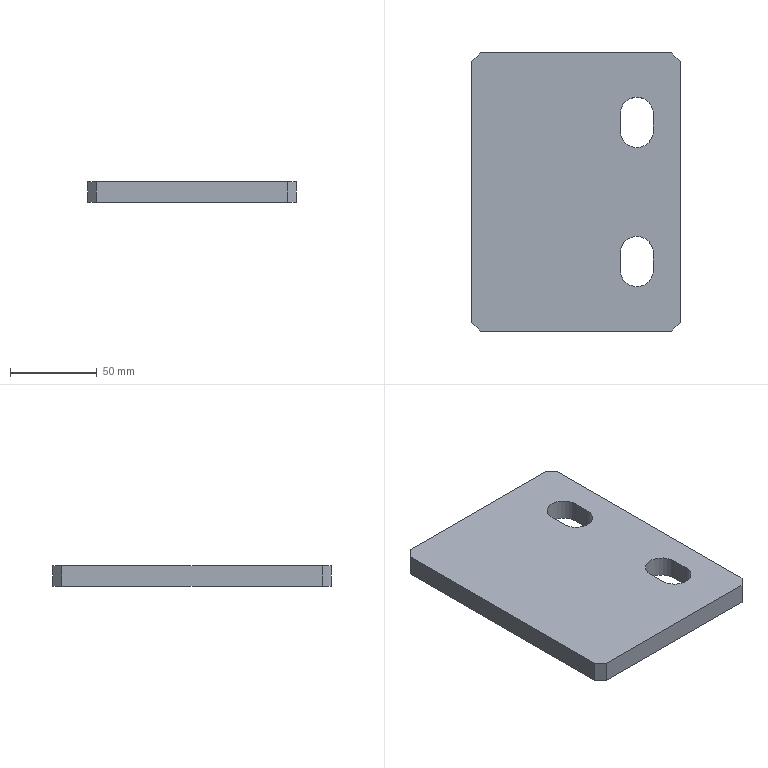Part | STEP file | Mirror_楼梯连接Plate 11 | 1 solid | 18 faces | box 120 x 160 x 12 mm | volume 218435 mm3 | plane 14 | cylinder 4 | commonest cylinder face diameters 19 x4
STEP:
#1=CARTESIAN_POINT('',(0.,0.,0.));
#2=DIRECTION('',(0.,0.,1.));
#3=DIRECTION('',(1.,0.,0.));
#4=AXIS2_PLACEMENT_3D('',#1,#2,#3);
#5=CARTESIAN_POINT('',(-60.,155.,0.));
#6=VERTEX_POINT('',#5);
#7=CARTESIAN_POINT('',(-60.,5.,0.));
#8=VERTEX_POINT('',#7);
#9=CARTESIAN_POINT('',(-60.,160.,0.));
#10=DIRECTION('',(0.,-1.,0.));
#11=VECTOR('',#10,1.);
#12=LINE('',#9,#11);
#13=CARTESIAN_POINT('',(-60.,160.,-12.));
#14=DIRECTION('',(1.,0.,0.));
#15=DIRECTION('',(0.,1.,0.));
#16=AXIS2_PLACEMENT_3D('',#13,#14,#15);
#17=PLANE('',#16);
#18=CARTESIAN_POINT('',(0.,12.));
#19=DIRECTION('',(-1.,0.));
#20=VECTOR('',#19,1.);
#21=LINE('',#18,#20);
#22=(GEOMETRIC_REPRESENTATION_CONTEXT(2)PARAMETRIC_REPRESENTATION_CONTEXT()REPRESENTATION_CONTEXT('',''));
#23=DEFINITIONAL_REPRESENTATION('',(#21),#22);
#24=PCURVE('',#17,#23);
#25=CARTESIAN_POINT('',(0.,0.,0.));
#26=DIRECTION('',(0.,0.,-1.));
#27=DIRECTION('',(1.,0.,0.));
#28=AXIS2_PLACEMENT_3D('',#25,#26,#27);
#29=PLANE('',#28);
#30=CARTESIAN_POINT('',(-60.,-160.));
#31=DIRECTION('',(0.,1.));
#32=VECTOR('',#31,1.);
#33=LINE('',#30,#32);
#34=(GEOMETRIC_REPRESENTATION_CONTEXT(2)PARAMETRIC_REPRESENTATION_CONTEXT()REPRESENTATION_CONTEXT('',''));
#35=DEFINITIONAL_REPRESENTATION('',(#33),#34);
#36=PCURVE('',#29,#35);
#37=SURFACE_CURVE('',#12,(#24,#36),.PCURVE_S1.);
#38=EDGE_CURVE('',#6,#8,#37,.T.);
#39=ORIENTED_EDGE('',*,*,#38,.F.);
#40=CARTESIAN_POINT('',(-60.,155.,-12.));
#41=VERTEX_POINT('',#40);
#42=CARTESIAN_POINT('',(-60.,155.,-12.));
#43=DIRECTION('',(0.,0.,1.));
#44=VECTOR('',#43,1.);
#45=LINE('',#42,#44);
#46=CARTESIAN_POINT('',(-5.,0.));
#47=DIRECTION('',(0.,1.));
#48=VECTOR('',#47,1.);
#49=LINE('',#46,#48);
#50=(GEOMETRIC_REPRESENTATION_CONTEXT(2)PARAMETRIC_REPRESENTATION_CONTEXT()REPRESENTATION_CONTEXT('',''));
#51=DEFINITIONAL_REPRESENTATION('',(#49),#50);
#52=PCURVE('',#17,#51);
#53=CARTESIAN_POINT('',(-60.,155.,-12.));
#54=DIRECTION('',(0.7071,-0.7071,0.));
#55=DIRECTION('',(0.,0.,1.));
#56=AXIS2_PLACEMENT_3D('',#53,#54,#55);
#57=PLANE('',#56);
#58=CARTESIAN_POINT('',(0.,0.));
#59=DIRECTION('',(1.,0.));
#60=VECTOR('',#59,1.);
#61=LINE('',#58,#60);
#62=(GEOMETRIC_REPRESENTATION_CONTEXT(2)PARAMETRIC_REPRESENTATION_CONTEXT()REPRESENTATION_CONTEXT('',''));
#63=DEFINITIONAL_REPRESENTATION('',(#61),#62);
#64=PCURVE('',#57,#63);
#65=SURFACE_CURVE('',#45,(#52,#64),.PCURVE_S1.);
#66=EDGE_CURVE('',#41,#6,#65,.T.);
#67=ORIENTED_EDGE('',*,*,#66,.F.);
#68=CARTESIAN_POINT('',(-60.,5.,-12.));
#69=VERTEX_POINT('',#68);
#70=CARTESIAN_POINT('',(-60.,160.,-12.));
#71=DIRECTION('',(0.,-1.,0.));
#72=VECTOR('',#71,1.);
#73=LINE('',#70,#72);
#74=CARTESIAN_POINT('',(0.,0.));
#75=DIRECTION('',(-1.,0.));
#76=VECTOR('',#75,1.);
#77=LINE('',#74,#76);
#78=(GEOMETRIC_REPRESENTATION_CONTEXT(2)PARAMETRIC_REPRESENTATION_CONTEXT()REPRESENTATION_CONTEXT('',''));
#79=DEFINITIONAL_REPRESENTATION('',(#77),#78);
#80=PCURVE('',#17,#79);
#81=CARTESIAN_POINT('',(0.,0.,-12.));
#82=DIRECTION('',(0.,0.,-1.));
#83=DIRECTION('',(1.,0.,0.));
#84=AXIS2_PLACEMENT_3D('',#81,#82,#83);
#85=PLANE('',#84);
#86=CARTESIAN_POINT('',(-60.,-160.));
#87=DIRECTION('',(0.,1.));
#88=VECTOR('',#87,1.);
#89=LINE('',#86,#88);
#90=(GEOMETRIC_REPRESENTATION_CONTEXT(2)PARAMETRIC_REPRESENTATION_CONTEXT()REPRESENTATION_CONTEXT('',''));
#91=DEFINITIONAL_REPRESENTATION('',(#89),#90);
#92=PCURVE('',#85,#91);
#93=SURFACE_CURVE('',#73,(#80,#92),.PCURVE_S1.);
#94=EDGE_CURVE('',#41,#69,#93,.T.);
#95=ORIENTED_EDGE('',*,*,#94,.T.);
#96=CARTESIAN_POINT('',(-60.,5.,-12.));
#97=DIRECTION('',(0.,0.,-1.));
#98=VECTOR('',#97,1.);
#99=LINE('',#96,#98);
#100=CARTESIAN_POINT('',(-155.,0.));
#101=DIRECTION('',(0.,-1.));
#102=VECTOR('',#101,1.);
#103=LINE('',#100,#102);
#104=(GEOMETRIC_REPRESENTATION_CONTEXT(2)PARAMETRIC_REPRESENTATION_CONTEXT()REPRESENTATION_CONTEXT('',''));
#105=DEFINITIONAL_REPRESENTATION('',(#103),#104);
#106=PCURVE('',#17,#105);
#107=CARTESIAN_POINT('',(-55.,0.,-12.));
#108=DIRECTION('',(0.7071,0.7071,0.));
#109=DIRECTION('',(0.,0.,1.));
#110=AXIS2_PLACEMENT_3D('',#107,#108,#109);
#111=PLANE('',#110);
#112=CARTESIAN_POINT('',(0.,-7.071));
#113=DIRECTION('',(-1.,0.));
#114=VECTOR('',#113,1.);
#115=LINE('',#112,#114);
#116=(GEOMETRIC_REPRESENTATION_CONTEXT(2)PARAMETRIC_REPRESENTATION_CONTEXT()REPRESENTATION_CONTEXT('',''));
#117=DEFINITIONAL_REPRESENTATION('',(#115),#116);
#118=PCURVE('',#111,#117);
#119=SURFACE_CURVE('',#99,(#106,#118),.PCURVE_S1.);
#120=EDGE_CURVE('',#8,#69,#119,.T.);
#121=ORIENTED_EDGE('',*,*,#120,.F.);
#122=EDGE_LOOP('',(#39,#67,#95,#121));
#123=FACE_BOUND('',#122,.T.);
#124=ADVANCED_FACE('',(#123),#17,.F.);
#125=CARTESIAN_POINT('',(-55.,0.,-12.));
#126=VERTEX_POINT('',#125);
#127=CARTESIAN_POINT('',(55.,0.,-12.));
#128=VERTEX_POINT('',#127);
#129=CARTESIAN_POINT('',(-60.,0.,-12.));
#130=DIRECTION('',(1.,0.,0.));
#131=VECTOR('',#130,1.);
#132=LINE('',#129,#131);
#133=CARTESIAN_POINT('',(-60.,0.,-12.));
#134=DIRECTION('',(0.,1.,0.));
#135=DIRECTION('',(0.,0.,-1.));
#136=AXIS2_PLACEMENT_3D('',#133,#134,#135);
#137=PLANE('',#136);
#138=CARTESIAN_POINT('',(0.,0.));
#139=DIRECTION('',(0.,-1.));
#140=VECTOR('',#139,1.);
#141=LINE('',#138,#140);
#142=(GEOMETRIC_REPRESENTATION_CONTEXT(2)PARAMETRIC_REPRESENTATION_CONTEXT()REPRESENTATION_CONTEXT('',''));
#143=DEFINITIONAL_REPRESENTATION('',(#141),#142);
#144=PCURVE('',#137,#143);
#145=CARTESIAN_POINT('',(-60.,0.));
#146=DIRECTION('',(1.,0.));
#147=VECTOR('',#146,1.);
#148=LINE('',#145,#147);
#149=(GEOMETRIC_REPRESENTATION_CONTEXT(2)PARAMETRIC_REPRESENTATION_CONTEXT()REPRESENTATION_CONTEXT('',''));
#150=DEFINITIONAL_REPRESENTATION('',(#148),#149);
#151=PCURVE('',#85,#150);
#152=SURFACE_CURVE('',#132,(#144,#151),.PCURVE_S1.);
#153=EDGE_CURVE('',#126,#128,#152,.T.);
#154=ORIENTED_EDGE('',*,*,#153,.T.);
#155=CARTESIAN_POINT('',(55.,0.,0.));
#156=VERTEX_POINT('',#155);
#157=CARTESIAN_POINT('',(55.,0.,-12.));
#158=DIRECTION('',(0.,0.,-1.));
#159=VECTOR('',#158,1.);
#160=LINE('',#157,#159);
#161=CARTESIAN_POINT('',(0.,-115.));
#162=DIRECTION('',(1.,0.));
#163=VECTOR('',#162,1.);
#164=LINE('',#161,#163);
#165=(GEOMETRIC_REPRESENTATION_CONTEXT(2)PARAMETRIC_REPRESENTATION_CONTEXT()REPRESENTATION_CONTEXT('',''));
#166=DEFINITIONAL_REPRESENTATION('',(#164),#165);
#167=PCURVE('',#137,#166);
#168=CARTESIAN_POINT('',(60.,5.,-12.));
#169=DIRECTION('',(-0.7071,0.7071,0.));
#170=DIRECTION('',(0.,0.,1.));
#171=AXIS2_PLACEMENT_3D('',#168,#169,#170);
#172=PLANE('',#171);
#173=CARTESIAN_POINT('',(0.,-7.071));
#174=DIRECTION('',(-1.,0.));
#175=VECTOR('',#174,1.);
#176=LINE('',#173,#175);
#177=(GEOMETRIC_REPRESENTATION_CONTEXT(2)PARAMETRIC_REPRESENTATION_CONTEXT()REPRESENTATION_CONTEXT('',''));
#178=DEFINITIONAL_REPRESENTATION('',(#176),#177);
#179=PCURVE('',#172,#178);
#180=SURFACE_CURVE('',#160,(#167,#179),.PCURVE_S1.);
#181=EDGE_CURVE('',#156,#128,#180,.T.);
#182=ORIENTED_EDGE('',*,*,#181,.F.);
#183=CARTESIAN_POINT('',(-55.,0.,0.));
#184=VERTEX_POINT('',#183);
#185=CARTESIAN_POINT('',(-60.,0.,0.));
#186=DIRECTION('',(1.,0.,0.));
#187=VECTOR('',#186,1.);
#188=LINE('',#185,#187);
#189=CARTESIAN_POINT('',(-12.,0.));
#190=DIRECTION('',(0.,-1.));
#191=VECTOR('',#190,1.);
#192=LINE('',#189,#191);
#193=(GEOMETRIC_REPRESENTATION_CONTEXT(2)PARAMETRIC_REPRESENTATION_CONTEXT()REPRESENTATION_CONTEXT('',''));
#194=DEFINITIONAL_REPRESENTATION('',(#192),#193);
#195=PCURVE('',#137,#194);
#196=CARTESIAN_POINT('',(-60.,0.));
#197=DIRECTION('',(1.,0.));
#198=VECTOR('',#197,1.);
#199=LINE('',#196,#198);
#200=(GEOMETRIC_REPRESENTATION_CONTEXT(2)PARAMETRIC_REPRESENTATION_CONTEXT()REPRESENTATION_CONTEXT('',''));
#201=DEFINITIONAL_REPRESENTATION('',(#199),#200);
#202=PCURVE('',#29,#201);
#203=SURFACE_CURVE('',#188,(#195,#202),.PCURVE_S1.);
#204=EDGE_CURVE('',#184,#156,#203,.T.);
#205=ORIENTED_EDGE('',*,*,#204,.F.);
#206=CARTESIAN_POINT('',(-55.,0.,-12.));
#207=DIRECTION('',(0.,0.,1.));
#208=VECTOR('',#207,1.);
#209=LINE('',#206,#208);
#210=CARTESIAN_POINT('',(0.,-5.));
#211=DIRECTION('',(-1.,0.));
#212=VECTOR('',#211,1.);
#213=LINE('',#210,#212);
#214=(GEOMETRIC_REPRESENTATION_CONTEXT(2)PARAMETRIC_REPRESENTATION_CONTEXT()REPRESENTATION_CONTEXT('',''));
#215=DEFINITIONAL_REPRESENTATION('',(#213),#214);
#216=PCURVE('',#137,#215);
#217=CARTESIAN_POINT('',(0.,0.));
#218=DIRECTION('',(1.,0.));
#219=VECTOR('',#218,1.);
#220=LINE('',#217,#219);
#221=(GEOMETRIC_REPRESENTATION_CONTEXT(2)PARAMETRIC_REPRESENTATION_CONTEXT()REPRESENTATION_CONTEXT('',''));
#222=DEFINITIONAL_REPRESENTATION('',(#220),#221);
#223=PCURVE('',#111,#222);
#224=SURFACE_CURVE('',#209,(#216,#223),.PCURVE_S1.);
#225=EDGE_CURVE('',#126,#184,#224,.T.);
#226=ORIENTED_EDGE('',*,*,#225,.F.);
#227=EDGE_LOOP('',(#154,#182,#205,#226));
#228=FACE_BOUND('',#227,.T.);
#229=ADVANCED_FACE('',(#228),#137,.F.);
#230=CARTESIAN_POINT('',(60.,5.,-12.));
#231=VERTEX_POINT('',#230);
#232=CARTESIAN_POINT('',(60.,155.,-12.));
#233=VERTEX_POINT('',#232);
#234=CARTESIAN_POINT('',(60.,160.,-12.));
#235=DIRECTION('',(0.,1.,0.));
#236=VECTOR('',#235,1.);
#237=LINE('',#234,#236);
#238=CARTESIAN_POINT('',(60.,160.,-12.));
#239=DIRECTION('',(-1.,0.,0.));
#240=DIRECTION('',(0.,-1.,0.));
#241=AXIS2_PLACEMENT_3D('',#238,#239,#240);
#242=PLANE('',#241);
#243=CARTESIAN_POINT('',(0.,0.));
#244=DIRECTION('',(-1.,0.));
#245=VECTOR('',#244,1.);
#246=LINE('',#243,#245);
#247=(GEOMETRIC_REPRESENTATION_CONTEXT(2)PARAMETRIC_REPRESENTATION_CONTEXT()REPRESENTATION_CONTEXT('',''));
#248=DEFINITIONAL_REPRESENTATION('',(#246),#247);
#249=PCURVE('',#242,#248);
#250=CARTESIAN_POINT('',(60.,-160.));
#251=DIRECTION('',(0.,-1.));
#252=VECTOR('',#251,1.);
#253=LINE('',#250,#252);
#254=(GEOMETRIC_REPRESENTATION_CONTEXT(2)PARAMETRIC_REPRESENTATION_CONTEXT()REPRESENTATION_CONTEXT('',''));
#255=DEFINITIONAL_REPRESENTATION('',(#253),#254);
#256=PCURVE('',#85,#255);
#257=SURFACE_CURVE('',#237,(#249,#256),.PCURVE_S1.);
#258=EDGE_CURVE('',#231,#233,#257,.T.);
#259=ORIENTED_EDGE('',*,*,#258,.T.);
#260=CARTESIAN_POINT('',(60.,155.,0.));
#261=VERTEX_POINT('',#260);
#262=CARTESIAN_POINT('',(60.,155.,-12.));
#263=DIRECTION('',(0.,0.,-1.));
#264=VECTOR('',#263,1.);
#265=LINE('',#262,#264);
#266=CARTESIAN_POINT('',(5.,0.));
#267=DIRECTION('',(0.,-1.));
#268=VECTOR('',#267,1.);
#269=LINE('',#266,#268);
#270=(GEOMETRIC_REPRESENTATION_CONTEXT(2)PARAMETRIC_REPRESENTATION_CONTEXT()REPRESENTATION_CONTEXT('',''));
#271=DEFINITIONAL_REPRESENTATION('',(#269),#270);
#272=PCURVE('',#242,#271);
#273=CARTESIAN_POINT('',(55.,160.,-12.));
#274=DIRECTION('',(-0.7071,-0.7071,0.));
#275=DIRECTION('',(0.,0.,1.));
#276=AXIS2_PLACEMENT_3D('',#273,#274,#275);
#277=PLANE('',#276);
#278=CARTESIAN_POINT('',(0.,-7.071));
#279=DIRECTION('',(-1.,0.));
#280=VECTOR('',#279,1.);
#281=LINE('',#278,#280);
#282=(GEOMETRIC_REPRESENTATION_CONTEXT(2)PARAMETRIC_REPRESENTATION_CONTEXT()REPRESENTATION_CONTEXT('',''));
#283=DEFINITIONAL_REPRESENTATION('',(#281),#282);
#284=PCURVE('',#277,#283);
#285=SURFACE_CURVE('',#265,(#272,#284),.PCURVE_S1.);
#286=EDGE_CURVE('',#261,#233,#285,.T.);
#287=ORIENTED_EDGE('',*,*,#286,.F.);
#288=CARTESIAN_POINT('',(60.,5.,0.));
#289=VERTEX_POINT('',#288);
#290=CARTESIAN_POINT('',(60.,160.,0.));
#291=DIRECTION('',(0.,1.,0.));
#292=VECTOR('',#291,1.);
#293=LINE('',#290,#292);
#294=CARTESIAN_POINT('',(0.,12.));
#295=DIRECTION('',(-1.,0.));
#296=VECTOR('',#295,1.);
#297=LINE('',#294,#296);
#298=(GEOMETRIC_REPRESENTATION_CONTEXT(2)PARAMETRIC_REPRESENTATION_CONTEXT()REPRESENTATION_CONTEXT('',''));
#299=DEFINITIONAL_REPRESENTATION('',(#297),#298);
#300=PCURVE('',#242,#299);
#301=CARTESIAN_POINT('',(60.,-160.));
#302=DIRECTION('',(0.,-1.));
#303=VECTOR('',#302,1.);
#304=LINE('',#301,#303);
#305=(GEOMETRIC_REPRESENTATION_CONTEXT(2)PARAMETRIC_REPRESENTATION_CONTEXT()REPRESENTATION_CONTEXT('',''));
#306=DEFINITIONAL_REPRESENTATION('',(#304),#305);
#307=PCURVE('',#29,#306);
#308=SURFACE_CURVE('',#293,(#300,#307),.PCURVE_S1.);
#309=EDGE_CURVE('',#289,#261,#308,.T.);
#310=ORIENTED_EDGE('',*,*,#309,.F.);
#311=CARTESIAN_POINT('',(60.,5.,-12.));
#312=DIRECTION('',(0.,0.,1.));
#313=VECTOR('',#312,1.);
#314=LINE('',#311,#313);
#315=CARTESIAN_POINT('',(155.,0.));
#316=DIRECTION('',(0.,1.));
#317=VECTOR('',#316,1.);
#318=LINE('',#315,#317);
#319=(GEOMETRIC_REPRESENTATION_CONTEXT(2)PARAMETRIC_REPRESENTATION_CONTEXT()REPRESENTATION_CONTEXT('',''));
#320=DEFINITIONAL_REPRESENTATION('',(#318),#319);
#321=PCURVE('',#242,#320);
#322=CARTESIAN_POINT('',(0.,0.));
#323=DIRECTION('',(1.,0.));
#324=VECTOR('',#323,1.);
#325=LINE('',#322,#324);
#326=(GEOMETRIC_REPRESENTATION_CONTEXT(2)PARAMETRIC_REPRESENTATION_CONTEXT()REPRESENTATION_CONTEXT('',''));
#327=DEFINITIONAL_REPRESENTATION('',(#325),#326);
#328=PCURVE('',#172,#327);
#329=SURFACE_CURVE('',#314,(#321,#328),.PCURVE_S1.);
#330=EDGE_CURVE('',#231,#289,#329,.T.);
#331=ORIENTED_EDGE('',*,*,#330,.F.);
#332=EDGE_LOOP('',(#259,#287,#310,#331));
#333=FACE_BOUND('',#332,.T.);
#334=ADVANCED_FACE('',(#333),#242,.F.);
#335=CARTESIAN_POINT('',(55.,160.,-12.));
#336=VERTEX_POINT('',#335);
#337=CARTESIAN_POINT('',(-55.,160.,-12.));
#338=VERTEX_POINT('',#337);
#339=CARTESIAN_POINT('',(-60.,160.,-12.));
#340=DIRECTION('',(-1.,0.,0.));
#341=VECTOR('',#340,1.);
#342=LINE('',#339,#341);
#343=CARTESIAN_POINT('',(-60.,160.,-12.));
#344=DIRECTION('',(0.,-1.,0.));
#345=DIRECTION('',(0.,0.,1.));
#346=AXIS2_PLACEMENT_3D('',#343,#344,#345);
#347=PLANE('',#346);
#348=CARTESIAN_POINT('',(0.,0.));
#349=DIRECTION('',(0.,1.));
#350=VECTOR('',#349,1.);
#351=LINE('',#348,#350);
#352=(GEOMETRIC_REPRESENTATION_CONTEXT(2)PARAMETRIC_REPRESENTATION_CONTEXT()REPRESENTATION_CONTEXT('',''));
#353=DEFINITIONAL_REPRESENTATION('',(#351),#352);
#354=PCURVE('',#347,#353);
#355=CARTESIAN_POINT('',(-60.,-160.));
#356=DIRECTION('',(-1.,0.));
#357=VECTOR('',#356,1.);
#358=LINE('',#355,#357);
#359=(GEOMETRIC_REPRESENTATION_CONTEXT(2)PARAMETRIC_REPRESENTATION_CONTEXT()REPRESENTATION_CONTEXT('',''));
#360=DEFINITIONAL_REPRESENTATION('',(#358),#359);
#361=PCURVE('',#85,#360);
#362=SURFACE_CURVE('',#342,(#354,#361),.PCURVE_S1.);
#363=EDGE_CURVE('',#336,#338,#362,.T.);
#364=ORIENTED_EDGE('',*,*,#363,.T.);
#365=CARTESIAN_POINT('',(-55.,160.,0.));
#366=VERTEX_POINT('',#365);
#367=CARTESIAN_POINT('',(-55.,160.,-12.));
#368=DIRECTION('',(0.,0.,-1.));
#369=VECTOR('',#368,1.);
#370=LINE('',#367,#369);
#371=CARTESIAN_POINT('',(0.,-5.));
#372=DIRECTION('',(-1.,0.));
#373=VECTOR('',#372,1.);
#374=LINE('',#371,#373);
#375=(GEOMETRIC_REPRESENTATION_CONTEXT(2)PARAMETRIC_REPRESENTATION_CONTEXT()REPRESENTATION_CONTEXT('',''));
#376=DEFINITIONAL_REPRESENTATION('',(#374),#375);
#377=PCURVE('',#347,#376);
#378=CARTESIAN_POINT('',(0.,-7.071));
#379=DIRECTION('',(-1.,0.));
#380=VECTOR('',#379,1.);
#381=LINE('',#378,#380);
#382=(GEOMETRIC_REPRESENTATION_CONTEXT(2)PARAMETRIC_REPRESENTATION_CONTEXT()REPRESENTATION_CONTEXT('',''));
#383=DEFINITIONAL_REPRESENTATION('',(#381),#382);
#384=PCURVE('',#57,#383);
#385=SURFACE_CURVE('',#370,(#377,#384),.PCURVE_S1.);
#386=EDGE_CURVE('',#366,#338,#385,.T.);
#387=ORIENTED_EDGE('',*,*,#386,.F.);
#388=CARTESIAN_POINT('',(55.,160.,0.));
#389=VERTEX_POINT('',#388);
#390=CARTESIAN_POINT('',(-60.,160.,0.));
#391=DIRECTION('',(-1.,0.,0.));
#392=VECTOR('',#391,1.);
#393=LINE('',#390,#392);
#394=CARTESIAN_POINT('',(12.,0.));
#395=DIRECTION('',(0.,1.));
#396=VECTOR('',#395,1.);
#397=LINE('',#394,#396);
#398=(GEOMETRIC_REPRESENTATION_CONTEXT(2)PARAMETRIC_REPRESENTATION_CONTEXT()REPRESENTATION_CONTEXT('',''));
#399=DEFINITIONAL_REPRESENTATION('',(#397),#398);
#400=PCURVE('',#347,#399);
#401=CARTESIAN_POINT('',(-60.,-160.));
#402=DIRECTION('',(-1.,0.));
#403=VECTOR('',#402,1.);
#404=LINE('',#401,#403);
#405=(GEOMETRIC_REPRESENTATION_CONTEXT(2)PARAMETRIC_REPRESENTATION_CONTEXT()REPRESENTATION_CONTEXT('',''));
#406=DEFINITIONAL_REPRESENTATION('',(#404),#405);
#407=PCURVE('',#29,#406);
#408=SURFACE_CURVE('',#393,(#400,#407),.PCURVE_S1.);
#409=EDGE_CURVE('',#389,#366,#408,.T.);
#410=ORIENTED_EDGE('',*,*,#409,.F.);
#411=CARTESIAN_POINT('',(55.,160.,-12.));
#412=DIRECTION('',(0.,0.,1.));
#413=VECTOR('',#412,1.);
#414=LINE('',#411,#413);
#415=CARTESIAN_POINT('',(0.,-115.));
#416=DIRECTION('',(1.,0.));
#417=VECTOR('',#416,1.);
#418=LINE('',#415,#417);
#419=(GEOMETRIC_REPRESENTATION_CONTEXT(2)PARAMETRIC_REPRESENTATION_CONTEXT()REPRESENTATION_CONTEXT('',''));
#420=DEFINITIONAL_REPRESENTATION('',(#418),#419);
#421=PCURVE('',#347,#420);
#422=CARTESIAN_POINT('',(0.,0.));
#423=DIRECTION('',(1.,0.));
#424=VECTOR('',#423,1.);
#425=LINE('',#422,#424);
#426=(GEOMETRIC_REPRESENTATION_CONTEXT(2)PARAMETRIC_REPRESENTATION_CONTEXT()REPRESENTATION_CONTEXT('',''));
#427=DEFINITIONAL_REPRESENTATION('',(#425),#426);
#428=PCURVE('',#277,#427);
#429=SURFACE_CURVE('',#414,(#421,#428),.PCURVE_S1.);
#430=EDGE_CURVE('',#336,#389,#429,.T.);
#431=ORIENTED_EDGE('',*,*,#430,.F.);
#432=EDGE_LOOP('',(#364,#387,#410,#431));
#433=FACE_BOUND('',#432,.T.);
#434=ADVANCED_FACE('',(#433),#347,.F.);
#435=CARTESIAN_POINT('',(44.5,115.,-12.));
#436=VERTEX_POINT('',#435);
#437=CARTESIAN_POINT('',(44.5,125.,-12.));
#438=VERTEX_POINT('',#437);
#439=CARTESIAN_POINT('',(44.5,115.,-12.));
#440=DIRECTION('',(0.,1.,0.));
#441=VECTOR('',#440,1.);
#442=LINE('',#439,#441);
#443=CARTESIAN_POINT('',(44.5,-115.));
#444=DIRECTION('',(0.,-1.));
#445=VECTOR('',#444,1.);
#446=LINE('',#443,#445);
#447=(GEOMETRIC_REPRESENTATION_CONTEXT(2)PARAMETRIC_REPRESENTATION_CONTEXT()REPRESENTATION_CONTEXT('',''));
#448=DEFINITIONAL_REPRESENTATION('',(#446),#447);
#449=PCURVE('',#85,#448);
#450=CARTESIAN_POINT('',(44.5,115.,0.001));
#451=DIRECTION('',(1.,0.,0.));
#452=DIRECTION('',(0.,0.,1.));
#453=AXIS2_PLACEMENT_3D('',#450,#451,#452);
#454=PLANE('',#453);
#455=CARTESIAN_POINT('',(-12.001,0.));
#456=DIRECTION('',(0.,-1.));
#457=VECTOR('',#456,1.);
#458=LINE('',#455,#457);
#459=(GEOMETRIC_REPRESENTATION_CONTEXT(2)PARAMETRIC_REPRESENTATION_CONTEXT()REPRESENTATION_CONTEXT('',''));
#460=DEFINITIONAL_REPRESENTATION('',(#458),#459);
#461=PCURVE('',#454,#460);
#462=SURFACE_CURVE('',#442,(#449,#461),.PCURVE_S1.);
#463=EDGE_CURVE('',#436,#438,#462,.T.);
#464=ORIENTED_EDGE('',*,*,#463,.T.);
#465=CARTESIAN_POINT('',(25.5,125.,-12.));
#466=VERTEX_POINT('',#465);
#467=CARTESIAN_POINT('',(35.,125.,-12.));
#468=DIRECTION('',(0.,0.,1.));
#469=DIRECTION('',(1.,0.,0.));
#470=AXIS2_PLACEMENT_3D('',#467,#468,#469);
#471=CIRCLE('',#470,9.5);
#472=CARTESIAN_POINT('',(44.5,-125.));
#473=CARTESIAN_POINT('',(44.5,-141.454));
#474=CARTESIAN_POINT('',(30.25,-133.227));
#475=CARTESIAN_POINT('',(16.,-125.));
#476=CARTESIAN_POINT('',(30.25,-116.773));
#477=CARTESIAN_POINT('',(44.5,-108.546));
#478=CARTESIAN_POINT('',(44.5,-125.));
#479=(BOUNDED_CURVE()B_SPLINE_CURVE(2,(#472,#473,#474,#475,#476,#477,#478),.UNSPECIFIED.,.T.,.F.)B_SPLINE_CURVE_WITH_KNOTS((1,2,2,2,2,1),(-2.094,0.,2.094,4.189,6.283,8.378),.UNSPECIFIED.)CURVE()GEOMETRIC_REPRESENTATION_ITEM()RATIONAL_B_SPLINE_CURVE((1.,0.5,1.,0.5,1.,0.5,1.))REPRESENTATION_ITEM(''));
#480=(GEOMETRIC_REPRESENTATION_CONTEXT(2)PARAMETRIC_REPRESENTATION_CONTEXT()REPRESENTATION_CONTEXT('',''));
#481=DEFINITIONAL_REPRESENTATION('',(#479),#480);
#482=PCURVE('',#85,#481);
#483=CARTESIAN_POINT('',(35.,125.,-12.));
#484=DIRECTION('',(0.,0.,-1.));
#485=DIRECTION('',(1.,0.,0.));
#486=AXIS2_PLACEMENT_3D('',#483,#484,#485);
#487=CYLINDRICAL_SURFACE('',#486,9.5);
#488=CARTESIAN_POINT('',(6.283,0.));
#489=DIRECTION('',(-1.,0.));
#490=VECTOR('',#489,1.);
#491=LINE('',#488,#490);
#492=(GEOMETRIC_REPRESENTATION_CONTEXT(2)PARAMETRIC_REPRESENTATION_CONTEXT()REPRESENTATION_CONTEXT('',''));
#493=DEFINITIONAL_REPRESENTATION('',(#491),#492);
#494=PCURVE('',#487,#493);
#495=SURFACE_CURVE('',#471,(#482,#494),.PCURVE_S1.);
#496=EDGE_CURVE('',#438,#466,#495,.T.);
#497=ORIENTED_EDGE('',*,*,#496,.T.);
#498=CARTESIAN_POINT('',(25.5,115.,-12.));
#499=VERTEX_POINT('',#498);
#500=CARTESIAN_POINT('',(25.5,115.,-12.));
#501=DIRECTION('',(0.,1.,0.));
#502=VECTOR('',#501,1.);
#503=LINE('',#500,#502);
#504=CARTESIAN_POINT('',(25.5,-115.));
#505=DIRECTION('',(0.,-1.));
#506=VECTOR('',#505,1.);
#507=LINE('',#504,#506);
#508=(GEOMETRIC_REPRESENTATION_CONTEXT(2)PARAMETRIC_REPRESENTATION_CONTEXT()REPRESENTATION_CONTEXT('',''));
#509=DEFINITIONAL_REPRESENTATION('',(#507),#508);
#510=PCURVE('',#85,#509);
#511=CARTESIAN_POINT('',(25.5,115.,-12.));
#512=DIRECTION('',(-1.,0.,0.));
#513=DIRECTION('',(0.,0.,-1.));
#514=AXIS2_PLACEMENT_3D('',#511,#512,#513);
#515=PLANE('',#514);
#516=CARTESIAN_POINT('',(0.,0.));
#517=DIRECTION('',(0.,-1.));
#518=VECTOR('',#517,1.);
#519=LINE('',#516,#518);
#520=(GEOMETRIC_REPRESENTATION_CONTEXT(2)PARAMETRIC_REPRESENTATION_CONTEXT()REPRESENTATION_CONTEXT('',''));
#521=DEFINITIONAL_REPRESENTATION('',(#519),#520);
#522=PCURVE('',#515,#521);
#523=SURFACE_CURVE('',#503,(#510,#522),.PCURVE_S1.);
#524=EDGE_CURVE('',#499,#466,#523,.T.);
#525=ORIENTED_EDGE('',*,*,#524,.F.);
#526=CARTESIAN_POINT('',(35.,115.,-12.));
#527=DIRECTION('',(0.,0.,1.));
#528=DIRECTION('',(1.,0.,0.));
#529=AXIS2_PLACEMENT_3D('',#526,#527,#528);
#530=CIRCLE('',#529,9.5);
#531=CARTESIAN_POINT('',(44.5,-115.));
#532=CARTESIAN_POINT('',(44.5,-131.454));
#533=CARTESIAN_POINT('',(30.25,-123.227));
#534=CARTESIAN_POINT('',(16.,-115.));
#535=CARTESIAN_POINT('',(30.25,-106.773));
#536=CARTESIAN_POINT('',(44.5,-98.546));
#537=CARTESIAN_POINT('',(44.5,-115.));
#538=(BOUNDED_CURVE()B_SPLINE_CURVE(2,(#531,#532,#533,#534,#535,#536,#537),.UNSPECIFIED.,.T.,.F.)B_SPLINE_CURVE_WITH_KNOTS((1,2,2,2,2,1),(-2.094,0.,2.094,4.189,6.283,8.378),.UNSPECIFIED.)CURVE()GEOMETRIC_REPRESENTATION_ITEM()RATIONAL_B_SPLINE_CURVE((1.,0.5,1.,0.5,1.,0.5,1.))REPRESENTATION_ITEM(''));
#539=(GEOMETRIC_REPRESENTATION_CONTEXT(2)PARAMETRIC_REPRESENTATION_CONTEXT()REPRESENTATION_CONTEXT('',''));
#540=DEFINITIONAL_REPRESENTATION('',(#538),#539);
#541=PCURVE('',#85,#540);
#542=CARTESIAN_POINT('',(35.,115.,-12.));
#543=DIRECTION('',(0.,0.,-1.));
#544=DIRECTION('',(1.,0.,0.));
#545=AXIS2_PLACEMENT_3D('',#542,#543,#544);
#546=CYLINDRICAL_SURFACE('',#545,9.5);
#547=CARTESIAN_POINT('',(6.283,0.));
#548=DIRECTION('',(-1.,0.));
#549=VECTOR('',#548,1.);
#550=LINE('',#547,#549);
#551=(GEOMETRIC_REPRESENTATION_CONTEXT(2)PARAMETRIC_REPRESENTATION_CONTEXT()REPRESENTATION_CONTEXT('',''));
#552=DEFINITIONAL_REPRESENTATION('',(#550),#551);
#553=PCURVE('',#546,#552);
#554=SURFACE_CURVE('',#530,(#541,#553),.PCURVE_S1.);
#555=EDGE_CURVE('',#499,#436,#554,.T.);
#556=ORIENTED_EDGE('',*,*,#555,.T.);
#557=EDGE_LOOP('',(#464,#497,#525,#556));
#558=FACE_BOUND('',#557,.T.);
#559=CARTESIAN_POINT('',(44.5,45.,-12.));
#560=VERTEX_POINT('',#559);
#561=CARTESIAN_POINT('',(25.5,45.,-12.));
#562=VERTEX_POINT('',#561);
#563=CARTESIAN_POINT('',(35.,45.,-12.));
#564=DIRECTION('',(0.,0.,1.));
#565=DIRECTION('',(1.,0.,0.));
#566=AXIS2_PLACEMENT_3D('',#563,#564,#565);
#567=CIRCLE('',#566,9.5);
#568=CARTESIAN_POINT('',(44.5,-45.));
#569=CARTESIAN_POINT('',(44.5,-61.454));
#570=CARTESIAN_POINT('',(30.25,-53.227));
#571=CARTESIAN_POINT('',(16.,-45.));
#572=CARTESIAN_POINT('',(30.25,-36.773));
#573=CARTESIAN_POINT('',(44.5,-28.546));
#574=CARTESIAN_POINT('',(44.5,-45.));
#575=(BOUNDED_CURVE()B_SPLINE_CURVE(2,(#568,#569,#570,#571,#572,#573,#574),.UNSPECIFIED.,.T.,.F.)B_SPLINE_CURVE_WITH_KNOTS((1,2,2,2,2,1),(-2.094,0.,2.094,4.189,6.283,8.378),.UNSPECIFIED.)CURVE()GEOMETRIC_REPRESENTATION_ITEM()RATIONAL_B_SPLINE_CURVE((1.,0.5,1.,0.5,1.,0.5,1.))REPRESENTATION_ITEM(''));
#576=(GEOMETRIC_REPRESENTATION_CONTEXT(2)PARAMETRIC_REPRESENTATION_CONTEXT()REPRESENTATION_CONTEXT('',''));
#577=DEFINITIONAL_REPRESENTATION('',(#575),#576);
#578=PCURVE('',#85,#577);
#579=CARTESIAN_POINT('',(35.,45.,-12.));
#580=DIRECTION('',(0.,0.,-1.));
#581=DIRECTION('',(1.,0.,0.));
#582=AXIS2_PLACEMENT_3D('',#579,#580,#581);
#583=CYLINDRICAL_SURFACE('',#582,9.5);
#584=CARTESIAN_POINT('',(6.283,0.));
#585=DIRECTION('',(-1.,0.));
#586=VECTOR('',#585,1.);
#587=LINE('',#584,#586);
#588=(GEOMETRIC_REPRESENTATION_CONTEXT(2)PARAMETRIC_REPRESENTATION_CONTEXT()REPRESENTATION_CONTEXT('',''));
#589=DEFINITIONAL_REPRESENTATION('',(#587),#588);
#590=PCURVE('',#583,#589);
#591=SURFACE_CURVE('',#567,(#578,#590),.PCURVE_S1.);
#592=EDGE_CURVE('',#560,#562,#591,.T.);
#593=ORIENTED_EDGE('',*,*,#592,.T.);
#594=CARTESIAN_POINT('',(25.5,35.,-12.));
#595=VERTEX_POINT('',#594);
#596=CARTESIAN_POINT('',(25.5,35.,-12.));
#597=DIRECTION('',(0.,1.,0.));
#598=VECTOR('',#597,1.);
#599=LINE('',#596,#598);
#600=CARTESIAN_POINT('',(25.5,-35.));
#601=DIRECTION('',(0.,-1.));
#602=VECTOR('',#601,1.);
#603=LINE('',#600,#602);
#604=(GEOMETRIC_REPRESENTATION_CONTEXT(2)PARAMETRIC_REPRESENTATION_CONTEXT()REPRESENTATION_CONTEXT('',''));
#605=DEFINITIONAL_REPRESENTATION('',(#603),#604);
#606=PCURVE('',#85,#605);
#607=CARTESIAN_POINT('',(25.5,35.,-12.));
#608=DIRECTION('',(-1.,0.,0.));
#609=DIRECTION('',(0.,0.,-1.));
#610=AXIS2_PLACEMENT_3D('',#607,#608,#609);
#611=PLANE('',#610);
#612=CARTESIAN_POINT('',(0.,0.));
#613=DIRECTION('',(0.,-1.));
#614=VECTOR('',#613,1.);
#615=LINE('',#612,#614);
#616=(GEOMETRIC_REPRESENTATION_CONTEXT(2)PARAMETRIC_REPRESENTATION_CONTEXT()REPRESENTATION_CONTEXT('',''));
#617=DEFINITIONAL_REPRESENTATION('',(#615),#616);
#618=PCURVE('',#611,#617);
#619=SURFACE_CURVE('',#599,(#606,#618),.PCURVE_S1.);
#620=EDGE_CURVE('',#595,#562,#619,.T.);
#621=ORIENTED_EDGE('',*,*,#620,.F.);
#622=CARTESIAN_POINT('',(44.5,35.,-12.));
#623=VERTEX_POINT('',#622);
#624=CARTESIAN_POINT('',(35.,35.,-12.));
#625=DIRECTION('',(0.,0.,1.));
#626=DIRECTION('',(1.,0.,0.));
#627=AXIS2_PLACEMENT_3D('',#624,#625,#626);
#628=CIRCLE('',#627,9.5);
#629=CARTESIAN_POINT('',(44.5,-35.));
#630=CARTESIAN_POINT('',(44.5,-51.454));
#631=CARTESIAN_POINT('',(30.25,-43.227));
#632=CARTESIAN_POINT('',(16.,-35.));
#633=CARTESIAN_POINT('',(30.25,-26.773));
#634=CARTESIAN_POINT('',(44.5,-18.546));
#635=CARTESIAN_POINT('',(44.5,-35.));
#636=(BOUNDED_CURVE()B_SPLINE_CURVE(2,(#629,#630,#631,#632,#633,#634,#635),.UNSPECIFIED.,.T.,.F.)B_SPLINE_CURVE_WITH_KNOTS((1,2,2,2,2,1),(-2.094,0.,2.094,4.189,6.283,8.378),.UNSPECIFIED.)CURVE()GEOMETRIC_REPRESENTATION_ITEM()RATIONAL_B_SPLINE_CURVE((1.,0.5,1.,0.5,1.,0.5,1.))REPRESENTATION_ITEM(''));
#637=(GEOMETRIC_REPRESENTATION_CONTEXT(2)PARAMETRIC_REPRESENTATION_CONTEXT()REPRESENTATION_CONTEXT('',''));
#638=DEFINITIONAL_REPRESENTATION('',(#636),#637);
#639=PCURVE('',#85,#638);
#640=CARTESIAN_POINT('',(35.,35.,-12.));
#641=DIRECTION('',(0.,0.,-1.));
#642=DIRECTION('',(1.,0.,0.));
#643=AXIS2_PLACEMENT_3D('',#640,#641,#642);
#644=CYLINDRICAL_SURFACE('',#643,9.5);
#645=CARTESIAN_POINT('',(6.283,0.));
#646=DIRECTION('',(-1.,0.));
#647=VECTOR('',#646,1.);
#648=LINE('',#645,#647);
#649=(GEOMETRIC_REPRESENTATION_CONTEXT(2)PARAMETRIC_REPRESENTATION_CONTEXT()REPRESENTATION_CONTEXT('',''));
#650=DEFINITIONAL_REPRESENTATION('',(#648),#649);
#651=PCURVE('',#644,#650);
#652=SURFACE_CURVE('',#628,(#639,#651),.PCURVE_S1.);
#653=EDGE_CURVE('',#595,#623,#652,.T.);
#654=ORIENTED_EDGE('',*,*,#653,.T.);
#655=CARTESIAN_POINT('',(44.5,35.,-12.));
#656=DIRECTION('',(0.,1.,0.));
#657=VECTOR('',#656,1.);
#658=LINE('',#655,#657);
#659=CARTESIAN_POINT('',(44.5,-35.));
#660=DIRECTION('',(0.,-1.));
#661=VECTOR('',#660,1.);
#662=LINE('',#659,#661);
#663=(GEOMETRIC_REPRESENTATION_CONTEXT(2)PARAMETRIC_REPRESENTATION_CONTEXT()REPRESENTATION_CONTEXT('',''));
#664=DEFINITIONAL_REPRESENTATION('',(#662),#663);
#665=PCURVE('',#85,#664);
#666=CARTESIAN_POINT('',(44.5,35.,0.001));
#667=DIRECTION('',(1.,0.,0.));
#668=DIRECTION('',(0.,0.,1.));
#669=AXIS2_PLACEMENT_3D('',#666,#667,#668);
#670=PLANE('',#669);
#671=CARTESIAN_POINT('',(-12.001,0.));
#672=DIRECTION('',(0.,-1.));
#673=VECTOR('',#672,1.);
#674=LINE('',#671,#673);
#675=(GEOMETRIC_REPRESENTATION_CONTEXT(2)PARAMETRIC_REPRESENTATION_CONTEXT()REPRESENTATION_CONTEXT('',''));
#676=DEFINITIONAL_REPRESENTATION('',(#674),#675);
#677=PCURVE('',#670,#676);
#678=SURFACE_CURVE('',#658,(#665,#677),.PCURVE_S1.);
#679=EDGE_CURVE('',#623,#560,#678,.T.);
#680=ORIENTED_EDGE('',*,*,#679,.T.);
#681=EDGE_LOOP('',(#593,#621,#654,#680));
#682=FACE_BOUND('',#681,.T.);
#683=ORIENTED_EDGE('',*,*,#94,.F.);
#684=CARTESIAN_POINT('',(-107.5,107.5,-12.));
#685=DIRECTION('',(-0.7071,-0.7071,0.));
#686=VECTOR('',#685,1.);
#687=LINE('',#684,#686);
#688=CARTESIAN_POINT('',(-107.5,-107.5));
#689=DIRECTION('',(-0.7071,0.7071));
#690=VECTOR('',#689,1.);
#691=LINE('',#688,#690);
#692=(GEOMETRIC_REPRESENTATION_CONTEXT(2)PARAMETRIC_REPRESENTATION_CONTEXT()REPRESENTATION_CONTEXT('',''));
#693=DEFINITIONAL_REPRESENTATION('',(#691),#692);
#694=PCURVE('',#85,#693);
#695=CARTESIAN_POINT('',(0.,67.175));
#696=DIRECTION('',(0.,1.));
#697=VECTOR('',#696,1.);
#698=LINE('',#695,#697);
#699=(GEOMETRIC_REPRESENTATION_CONTEXT(2)PARAMETRIC_REPRESENTATION_CONTEXT()REPRESENTATION_CONTEXT('',''));
#700=DEFINITIONAL_REPRESENTATION('',(#698),#699);
#701=PCURVE('',#57,#700);
#702=SURFACE_CURVE('',#687,(#694,#701),.PCURVE_S1.);
#703=EDGE_CURVE('',#338,#41,#702,.T.);
#704=ORIENTED_EDGE('',*,*,#703,.F.);
#705=ORIENTED_EDGE('',*,*,#363,.F.);
#706=CARTESIAN_POINT('',(107.5,107.5,-12.));
#707=DIRECTION('',(-0.7071,0.7071,0.));
#708=VECTOR('',#707,1.);
#709=LINE('',#706,#708);
#710=CARTESIAN_POINT('',(107.5,-107.5));
#711=DIRECTION('',(-0.7071,-0.7071));
#712=VECTOR('',#711,1.);
#713=LINE('',#710,#712);
#714=(GEOMETRIC_REPRESENTATION_CONTEXT(2)PARAMETRIC_REPRESENTATION_CONTEXT()REPRESENTATION_CONTEXT('',''));
#715=DEFINITIONAL_REPRESENTATION('',(#713),#714);
#716=PCURVE('',#85,#715);
#717=CARTESIAN_POINT('',(0.,-74.246));
#718=DIRECTION('',(0.,1.));
#719=VECTOR('',#718,1.);
#720=LINE('',#717,#719);
#721=(GEOMETRIC_REPRESENTATION_CONTEXT(2)PARAMETRIC_REPRESENTATION_CONTEXT()REPRESENTATION_CONTEXT('',''));
#722=DEFINITIONAL_REPRESENTATION('',(#720),#721);
#723=PCURVE('',#277,#722);
#724=SURFACE_CURVE('',#709,(#716,#723),.PCURVE_S1.);
#725=EDGE_CURVE('',#233,#336,#724,.T.);
#726=ORIENTED_EDGE('',*,*,#725,.F.);
#727=ORIENTED_EDGE('',*,*,#258,.F.);
#728=CARTESIAN_POINT('',(27.5,-27.5,-12.));
#729=DIRECTION('',(0.7071,0.7071,0.));
#730=VECTOR('',#729,1.);
#731=LINE('',#728,#730);
#732=CARTESIAN_POINT('',(27.5,27.5));
#733=DIRECTION('',(0.7071,-0.7071));
#734=VECTOR('',#733,1.);
#735=LINE('',#732,#734);
#736=(GEOMETRIC_REPRESENTATION_CONTEXT(2)PARAMETRIC_REPRESENTATION_CONTEXT()REPRESENTATION_CONTEXT('',''));
#737=DEFINITIONAL_REPRESENTATION('',(#735),#736);
#738=PCURVE('',#85,#737);
#739=CARTESIAN_POINT('',(0.,-45.962));
#740=DIRECTION('',(0.,1.));
#741=VECTOR('',#740,1.);
#742=LINE('',#739,#741);
#743=(GEOMETRIC_REPRESENTATION_CONTEXT(2)PARAMETRIC_REPRESENTATION_CONTEXT()REPRESENTATION_CONTEXT('',''));
#744=DEFINITIONAL_REPRESENTATION('',(#742),#743);
#745=PCURVE('',#172,#744);
#746=SURFACE_CURVE('',#731,(#738,#745),.PCURVE_S1.);
#747=EDGE_CURVE('',#128,#231,#746,.T.);
#748=ORIENTED_EDGE('',*,*,#747,.F.);
#749=ORIENTED_EDGE('',*,*,#153,.F.);
#750=CARTESIAN_POINT('',(-27.5,-27.5,-12.));
#751=DIRECTION('',(0.7071,-0.7071,0.));
#752=VECTOR('',#751,1.);
#753=LINE('',#750,#752);
#754=CARTESIAN_POINT('',(-27.5,27.5));
#755=DIRECTION('',(0.7071,0.7071));
#756=VECTOR('',#755,1.);
#757=LINE('',#754,#756);
#758=(GEOMETRIC_REPRESENTATION_CONTEXT(2)PARAMETRIC_REPRESENTATION_CONTEXT()REPRESENTATION_CONTEXT('',''));
#759=DEFINITIONAL_REPRESENTATION('',(#757),#758);
#760=PCURVE('',#85,#759);
#761=CARTESIAN_POINT('',(0.,38.891));
#762=DIRECTION('',(0.,1.));
#763=VECTOR('',#762,1.);
#764=LINE('',#761,#763);
#765=(GEOMETRIC_REPRESENTATION_CONTEXT(2)PARAMETRIC_REPRESENTATION_CONTEXT()REPRESENTATION_CONTEXT('',''));
#766=DEFINITIONAL_REPRESENTATION('',(#764),#765);
#767=PCURVE('',#111,#766);
#768=SURFACE_CURVE('',#753,(#760,#767),.PCURVE_S1.);
#769=EDGE_CURVE('',#69,#126,#768,.T.);
#770=ORIENTED_EDGE('',*,*,#769,.F.);
#771=EDGE_LOOP('',(#683,#704,#705,#726,#727,#748,#749,#770));
#772=FACE_BOUND('',#771,.T.);
#773=ADVANCED_FACE('',(#558,#682,#772),#85,.T.);
#774=CARTESIAN_POINT('',(44.5,125.,0.));
#775=VERTEX_POINT('',#774);
#776=CARTESIAN_POINT('',(25.5,125.,0.));
#777=VERTEX_POINT('',#776);
#778=CARTESIAN_POINT('',(35.,125.,0.));
#779=DIRECTION('',(0.,0.,1.));
#780=DIRECTION('',(1.,0.,0.));
#781=AXIS2_PLACEMENT_3D('',#778,#779,#780);
#782=CIRCLE('',#781,9.5);
#783=CARTESIAN_POINT('',(44.5,-125.));
#784=CARTESIAN_POINT('',(44.5,-141.454));
#785=CARTESIAN_POINT('',(30.25,-133.227));
#786=CARTESIAN_POINT('',(16.,-125.));
#787=CARTESIAN_POINT('',(30.25,-116.773));
#788=CARTESIAN_POINT('',(44.5,-108.546));
#789=CARTESIAN_POINT('',(44.5,-125.));
#790=(BOUNDED_CURVE()B_SPLINE_CURVE(2,(#783,#784,#785,#786,#787,#788,#789),.UNSPECIFIED.,.T.,.F.)B_SPLINE_CURVE_WITH_KNOTS((1,2,2,2,2,1),(-2.094,0.,2.094,4.189,6.283,8.378),.UNSPECIFIED.)CURVE()GEOMETRIC_REPRESENTATION_ITEM()RATIONAL_B_SPLINE_CURVE((1.,0.5,1.,0.5,1.,0.5,1.))REPRESENTATION_ITEM(''));
#791=(GEOMETRIC_REPRESENTATION_CONTEXT(2)PARAMETRIC_REPRESENTATION_CONTEXT()REPRESENTATION_CONTEXT('',''));
#792=DEFINITIONAL_REPRESENTATION('',(#790),#791);
#793=PCURVE('',#29,#792);
#794=CARTESIAN_POINT('',(6.283,-12.));
#795=DIRECTION('',(-1.,0.));
#796=VECTOR('',#795,1.);
#797=LINE('',#794,#796);
#798=(GEOMETRIC_REPRESENTATION_CONTEXT(2)PARAMETRIC_REPRESENTATION_CONTEXT()REPRESENTATION_CONTEXT('',''));
#799=DEFINITIONAL_REPRESENTATION('',(#797),#798);
#800=PCURVE('',#487,#799);
#801=SURFACE_CURVE('',#782,(#793,#800),.PCURVE_S1.);
#802=EDGE_CURVE('',#775,#777,#801,.T.);
#803=ORIENTED_EDGE('',*,*,#802,.F.);
#804=CARTESIAN_POINT('',(44.5,115.,0.));
#805=VERTEX_POINT('',#804);
#806=CARTESIAN_POINT('',(44.5,0.,0.));
#807=DIRECTION('',(0.,1.,0.));
#808=VECTOR('',#807,1.);
#809=LINE('',#806,#808);
#810=CARTESIAN_POINT('',(44.5,0.));
#811=DIRECTION('',(0.,-1.));
#812=VECTOR('',#811,1.);
#813=LINE('',#810,#812);
#814=(GEOMETRIC_REPRESENTATION_CONTEXT(2)PARAMETRIC_REPRESENTATION_CONTEXT()REPRESENTATION_CONTEXT('',''));
#815=DEFINITIONAL_REPRESENTATION('',(#813),#814);
#816=PCURVE('',#29,#815);
#817=CARTESIAN_POINT('',(-0.001,115.));
#818=DIRECTION('',(0.,-1.));
#819=VECTOR('',#818,1.);
#820=LINE('',#817,#819);
#821=(GEOMETRIC_REPRESENTATION_CONTEXT(2)PARAMETRIC_REPRESENTATION_CONTEXT()REPRESENTATION_CONTEXT('',''));
#822=DEFINITIONAL_REPRESENTATION('',(#820),#821);
#823=PCURVE('',#454,#822);
#824=SURFACE_CURVE('',#809,(#816,#823),.PCURVE_S1.);
#825=EDGE_CURVE('',#805,#775,#824,.T.);
#826=ORIENTED_EDGE('',*,*,#825,.F.);
#827=CARTESIAN_POINT('',(25.5,115.,0.));
#828=VERTEX_POINT('',#827);
#829=CARTESIAN_POINT('',(35.,115.,0.));
#830=DIRECTION('',(0.,0.,1.));
#831=DIRECTION('',(1.,0.,0.));
#832=AXIS2_PLACEMENT_3D('',#829,#830,#831);
#833=CIRCLE('',#832,9.5);
#834=CARTESIAN_POINT('',(44.5,-115.));
#835=CARTESIAN_POINT('',(44.5,-131.454));
#836=CARTESIAN_POINT('',(30.25,-123.227));
#837=CARTESIAN_POINT('',(16.,-115.));
#838=CARTESIAN_POINT('',(30.25,-106.773));
#839=CARTESIAN_POINT('',(44.5,-98.546));
#840=CARTESIAN_POINT('',(44.5,-115.));
#841=(BOUNDED_CURVE()B_SPLINE_CURVE(2,(#834,#835,#836,#837,#838,#839,#840),.UNSPECIFIED.,.T.,.F.)B_SPLINE_CURVE_WITH_KNOTS((1,2,2,2,2,1),(-2.094,0.,2.094,4.189,6.283,8.378),.UNSPECIFIED.)CURVE()GEOMETRIC_REPRESENTATION_ITEM()RATIONAL_B_SPLINE_CURVE((1.,0.5,1.,0.5,1.,0.5,1.))REPRESENTATION_ITEM(''));
#842=(GEOMETRIC_REPRESENTATION_CONTEXT(2)PARAMETRIC_REPRESENTATION_CONTEXT()REPRESENTATION_CONTEXT('',''));
#843=DEFINITIONAL_REPRESENTATION('',(#841),#842);
#844=PCURVE('',#29,#843);
#845=CARTESIAN_POINT('',(6.283,-12.));
#846=DIRECTION('',(-1.,0.));
#847=VECTOR('',#846,1.);
#848=LINE('',#845,#847);
#849=(GEOMETRIC_REPRESENTATION_CONTEXT(2)PARAMETRIC_REPRESENTATION_CONTEXT()REPRESENTATION_CONTEXT('',''));
#850=DEFINITIONAL_REPRESENTATION('',(#848),#849);
#851=PCURVE('',#546,#850);
#852=SURFACE_CURVE('',#833,(#844,#851),.PCURVE_S1.);
#853=EDGE_CURVE('',#828,#805,#852,.T.);
#854=ORIENTED_EDGE('',*,*,#853,.F.);
#855=CARTESIAN_POINT('',(25.5,0.,0.));
#856=DIRECTION('',(0.,-1.,0.));
#857=VECTOR('',#856,1.);
#858=LINE('',#855,#857);
#859=CARTESIAN_POINT('',(25.5,0.));
#860=DIRECTION('',(0.,1.));
#861=VECTOR('',#860,1.);
#862=LINE('',#859,#861);
#863=(GEOMETRIC_REPRESENTATION_CONTEXT(2)PARAMETRIC_REPRESENTATION_CONTEXT()REPRESENTATION_CONTEXT('',''));
#864=DEFINITIONAL_REPRESENTATION('',(#862),#863);
#865=PCURVE('',#29,#864);
#866=CARTESIAN_POINT('',(-12.,115.));
#867=DIRECTION('',(0.,1.));
#868=VECTOR('',#867,1.);
#869=LINE('',#866,#868);
#870=(GEOMETRIC_REPRESENTATION_CONTEXT(2)PARAMETRIC_REPRESENTATION_CONTEXT()REPRESENTATION_CONTEXT('',''));
#871=DEFINITIONAL_REPRESENTATION('',(#869),#870);
#872=PCURVE('',#515,#871);
#873=SURFACE_CURVE('',#858,(#865,#872),.PCURVE_S1.);
#874=EDGE_CURVE('',#777,#828,#873,.T.);
#875=ORIENTED_EDGE('',*,*,#874,.F.);
#876=EDGE_LOOP('',(#803,#826,#854,#875));
#877=FACE_BOUND('',#876,.T.);
#878=CARTESIAN_POINT('',(44.5,45.,0.));
#879=VERTEX_POINT('',#878);
#880=CARTESIAN_POINT('',(25.5,45.,0.));
#881=VERTEX_POINT('',#880);
#882=CARTESIAN_POINT('',(35.,45.,0.));
#883=DIRECTION('',(0.,0.,1.));
#884=DIRECTION('',(1.,0.,0.));
#885=AXIS2_PLACEMENT_3D('',#882,#883,#884);
#886=CIRCLE('',#885,9.5);
#887=CARTESIAN_POINT('',(44.5,-45.));
#888=CARTESIAN_POINT('',(44.5,-61.454));
#889=CARTESIAN_POINT('',(30.25,-53.227));
#890=CARTESIAN_POINT('',(16.,-45.));
#891=CARTESIAN_POINT('',(30.25,-36.773));
#892=CARTESIAN_POINT('',(44.5,-28.546));
#893=CARTESIAN_POINT('',(44.5,-45.));
#894=(BOUNDED_CURVE()B_SPLINE_CURVE(2,(#887,#888,#889,#890,#891,#892,#893),.UNSPECIFIED.,.T.,.F.)B_SPLINE_CURVE_WITH_KNOTS((1,2,2,2,2,1),(-2.094,0.,2.094,4.189,6.283,8.378),.UNSPECIFIED.)CURVE()GEOMETRIC_REPRESENTATION_ITEM()RATIONAL_B_SPLINE_CURVE((1.,0.5,1.,0.5,1.,0.5,1.))REPRESENTATION_ITEM(''));
#895=(GEOMETRIC_REPRESENTATION_CONTEXT(2)PARAMETRIC_REPRESENTATION_CONTEXT()REPRESENTATION_CONTEXT('',''));
#896=DEFINITIONAL_REPRESENTATION('',(#894),#895);
#897=PCURVE('',#29,#896);
#898=CARTESIAN_POINT('',(6.283,-12.));
#899=DIRECTION('',(-1.,0.));
#900=VECTOR('',#899,1.);
#901=LINE('',#898,#900);
#902=(GEOMETRIC_REPRESENTATION_CONTEXT(2)PARAMETRIC_REPRESENTATION_CONTEXT()REPRESENTATION_CONTEXT('',''));
#903=DEFINITIONAL_REPRESENTATION('',(#901),#902);
#904=PCURVE('',#583,#903);
#905=SURFACE_CURVE('',#886,(#897,#904),.PCURVE_S1.);
#906=EDGE_CURVE('',#879,#881,#905,.T.);
#907=ORIENTED_EDGE('',*,*,#906,.F.);
#908=CARTESIAN_POINT('',(44.5,35.,0.));
#909=VERTEX_POINT('',#908);
#910=CARTESIAN_POINT('',(44.5,0.,0.));
#911=DIRECTION('',(0.,1.,0.));
#912=VECTOR('',#911,1.);
#913=LINE('',#910,#912);
#914=CARTESIAN_POINT('',(44.5,0.));
#915=DIRECTION('',(0.,-1.));
#916=VECTOR('',#915,1.);
#917=LINE('',#914,#916);
#918=(GEOMETRIC_REPRESENTATION_CONTEXT(2)PARAMETRIC_REPRESENTATION_CONTEXT()REPRESENTATION_CONTEXT('',''));
#919=DEFINITIONAL_REPRESENTATION('',(#917),#918);
#920=PCURVE('',#29,#919);
#921=CARTESIAN_POINT('',(-0.001,35.));
#922=DIRECTION('',(0.,-1.));
#923=VECTOR('',#922,1.);
#924=LINE('',#921,#923);
#925=(GEOMETRIC_REPRESENTATION_CONTEXT(2)PARAMETRIC_REPRESENTATION_CONTEXT()REPRESENTATION_CONTEXT('',''));
#926=DEFINITIONAL_REPRESENTATION('',(#924),#925);
#927=PCURVE('',#670,#926);
#928=SURFACE_CURVE('',#913,(#920,#927),.PCURVE_S1.);
#929=EDGE_CURVE('',#909,#879,#928,.T.);
#930=ORIENTED_EDGE('',*,*,#929,.F.);
#931=CARTESIAN_POINT('',(25.5,35.,0.));
#932=VERTEX_POINT('',#931);
#933=CARTESIAN_POINT('',(35.,35.,0.));
#934=DIRECTION('',(0.,0.,1.));
#935=DIRECTION('',(1.,0.,0.));
#936=AXIS2_PLACEMENT_3D('',#933,#934,#935);
#937=CIRCLE('',#936,9.5);
#938=CARTESIAN_POINT('',(44.5,-35.));
#939=CARTESIAN_POINT('',(44.5,-51.454));
#940=CARTESIAN_POINT('',(30.25,-43.227));
#941=CARTESIAN_POINT('',(16.,-35.));
#942=CARTESIAN_POINT('',(30.25,-26.773));
#943=CARTESIAN_POINT('',(44.5,-18.546));
#944=CARTESIAN_POINT('',(44.5,-35.));
#945=(BOUNDED_CURVE()B_SPLINE_CURVE(2,(#938,#939,#940,#941,#942,#943,#944),.UNSPECIFIED.,.T.,.F.)B_SPLINE_CURVE_WITH_KNOTS((1,2,2,2,2,1),(-2.094,0.,2.094,4.189,6.283,8.378),.UNSPECIFIED.)CURVE()GEOMETRIC_REPRESENTATION_ITEM()RATIONAL_B_SPLINE_CURVE((1.,0.5,1.,0.5,1.,0.5,1.))REPRESENTATION_ITEM(''));
#946=(GEOMETRIC_REPRESENTATION_CONTEXT(2)PARAMETRIC_REPRESENTATION_CONTEXT()REPRESENTATION_CONTEXT('',''));
#947=DEFINITIONAL_REPRESENTATION('',(#945),#946);
#948=PCURVE('',#29,#947);
#949=CARTESIAN_POINT('',(6.283,-12.));
#950=DIRECTION('',(-1.,0.));
#951=VECTOR('',#950,1.);
#952=LINE('',#949,#951);
#953=(GEOMETRIC_REPRESENTATION_CONTEXT(2)PARAMETRIC_REPRESENTATION_CONTEXT()REPRESENTATION_CONTEXT('',''));
#954=DEFINITIONAL_REPRESENTATION('',(#952),#953);
#955=PCURVE('',#644,#954);
#956=SURFACE_CURVE('',#937,(#948,#955),.PCURVE_S1.);
#957=EDGE_CURVE('',#932,#909,#956,.T.);
#958=ORIENTED_EDGE('',*,*,#957,.F.);
#959=CARTESIAN_POINT('',(25.5,0.,0.));
#960=DIRECTION('',(0.,-1.,0.));
#961=VECTOR('',#960,1.);
#962=LINE('',#959,#961);
#963=CARTESIAN_POINT('',(25.5,0.));
#964=DIRECTION('',(0.,1.));
#965=VECTOR('',#964,1.);
#966=LINE('',#963,#965);
#967=(GEOMETRIC_REPRESENTATION_CONTEXT(2)PARAMETRIC_REPRESENTATION_CONTEXT()REPRESENTATION_CONTEXT('',''));
#968=DEFINITIONAL_REPRESENTATION('',(#966),#967);
#969=PCURVE('',#29,#968);
#970=CARTESIAN_POINT('',(-12.,35.));
#971=DIRECTION('',(0.,1.));
#972=VECTOR('',#971,1.);
#973=LINE('',#970,#972);
#974=(GEOMETRIC_REPRESENTATION_CONTEXT(2)PARAMETRIC_REPRESENTATION_CONTEXT()REPRESENTATION_CONTEXT('',''));
#975=DEFINITIONAL_REPRESENTATION('',(#973),#974);
#976=PCURVE('',#611,#975);
#977=SURFACE_CURVE('',#962,(#969,#976),.PCURVE_S1.);
#978=EDGE_CURVE('',#881,#932,#977,.T.);
#979=ORIENTED_EDGE('',*,*,#978,.F.);
#980=EDGE_LOOP('',(#907,#930,#958,#979));
#981=FACE_BOUND('',#980,.T.);
#982=ORIENTED_EDGE('',*,*,#204,.T.);
#983=CARTESIAN_POINT('',(60.,5.,0.));
#984=DIRECTION('',(-0.7071,-0.7071,0.));
#985=VECTOR('',#984,1.);
#986=LINE('',#983,#985);
#987=CARTESIAN_POINT('',(60.,-5.));
#988=DIRECTION('',(-0.7071,0.7071));
#989=VECTOR('',#988,1.);
#990=LINE('',#987,#989);
#991=(GEOMETRIC_REPRESENTATION_CONTEXT(2)PARAMETRIC_REPRESENTATION_CONTEXT()REPRESENTATION_CONTEXT('',''));
#992=DEFINITIONAL_REPRESENTATION('',(#990),#991);
#993=PCURVE('',#29,#992);
#994=CARTESIAN_POINT('',(12.,0.));
#995=DIRECTION('',(0.,-1.));
#996=VECTOR('',#995,1.);
#997=LINE('',#994,#996);
#998=(GEOMETRIC_REPRESENTATION_CONTEXT(2)PARAMETRIC_REPRESENTATION_CONTEXT()REPRESENTATION_CONTEXT('',''));
#999=DEFINITIONAL_REPRESENTATION('',(#997),#998);
#1000=PCURVE('',#172,#999);
#1001=SURFACE_CURVE('',#986,(#993,#1000),.PCURVE_S1.);
#1002=EDGE_CURVE('',#289,#156,#1001,.T.);
#1003=ORIENTED_EDGE('',*,*,#1002,.F.);
#1004=ORIENTED_EDGE('',*,*,#309,.T.);
#1005=CARTESIAN_POINT('',(55.,160.,0.));
#1006=DIRECTION('',(0.7071,-0.7071,0.));
#1007=VECTOR('',#1006,1.);
#1008=LINE('',#1005,#1007);
#1009=CARTESIAN_POINT('',(55.,-160.));
#1010=DIRECTION('',(0.7071,0.7071));
#1011=VECTOR('',#1010,1.);
#1012=LINE('',#1009,#1011);
#1013=(GEOMETRIC_REPRESENTATION_CONTEXT(2)PARAMETRIC_REPRESENTATION_CONTEXT()REPRESENTATION_CONTEXT('',''));
#1014=DEFINITIONAL_REPRESENTATION('',(#1012),#1013);
#1015=PCURVE('',#29,#1014);
#1016=CARTESIAN_POINT('',(12.,0.));
#1017=DIRECTION('',(0.,-1.));
#1018=VECTOR('',#1017,1.);
#1019=LINE('',#1016,#1018);
#1020=(GEOMETRIC_REPRESENTATION_CONTEXT(2)PARAMETRIC_REPRESENTATION_CONTEXT()REPRESENTATION_CONTEXT('',''));
#1021=DEFINITIONAL_REPRESENTATION('',(#1019),#1020);
#1022=PCURVE('',#277,#1021);
#1023=SURFACE_CURVE('',#1008,(#1015,#1022),.PCURVE_S1.);
#1024=EDGE_CURVE('',#389,#261,#1023,.T.);
#1025=ORIENTED_EDGE('',*,*,#1024,.F.);
#1026=ORIENTED_EDGE('',*,*,#409,.T.);
#1027=CARTESIAN_POINT('',(-60.,155.,0.));
#1028=DIRECTION('',(0.7071,0.7071,0.));
#1029=VECTOR('',#1028,1.);
#1030=LINE('',#1027,#1029);
#1031=CARTESIAN_POINT('',(-60.,-155.));
#1032=DIRECTION('',(0.7071,-0.7071));
#1033=VECTOR('',#1032,1.);
#1034=LINE('',#1031,#1033);
#1035=(GEOMETRIC_REPRESENTATION_CONTEXT(2)PARAMETRIC_REPRESENTATION_CONTEXT()REPRESENTATION_CONTEXT('',''));
#1036=DEFINITIONAL_REPRESENTATION('',(#1034),#1035);
#1037=PCURVE('',#29,#1036);
#1038=CARTESIAN_POINT('',(12.,0.));
#1039=DIRECTION('',(0.,-1.));
#1040=VECTOR('',#1039,1.);
#1041=LINE('',#1038,#1040);
#1042=(GEOMETRIC_REPRESENTATION_CONTEXT(2)PARAMETRIC_REPRESENTATION_CONTEXT()REPRESENTATION_CONTEXT('',''));
#1043=DEFINITIONAL_REPRESENTATION('',(#1041),#1042);
#1044=PCURVE('',#57,#1043);
#1045=SURFACE_CURVE('',#1030,(#1037,#1044),.PCURVE_S1.);
#1046=EDGE_CURVE('',#6,#366,#1045,.T.);
#1047=ORIENTED_EDGE('',*,*,#1046,.F.);
#1048=ORIENTED_EDGE('',*,*,#38,.T.);
#1049=CARTESIAN_POINT('',(-55.,0.,0.));
#1050=DIRECTION('',(-0.7071,0.7071,0.));
#1051=VECTOR('',#1050,1.);
#1052=LINE('',#1049,#1051);
#1053=CARTESIAN_POINT('',(-55.,0.));
#1054=DIRECTION('',(-0.7071,-0.7071));
#1055=VECTOR('',#1054,1.);
#1056=LINE('',#1053,#1055);
#1057=(GEOMETRIC_REPRESENTATION_CONTEXT(2)PARAMETRIC_REPRESENTATION_CONTEXT()REPRESENTATION_CONTEXT('',''));
#1058=DEFINITIONAL_REPRESENTATION('',(#1056),#1057);
#1059=PCURVE('',#29,#1058);
#1060=CARTESIAN_POINT('',(12.,0.));
#1061=DIRECTION('',(0.,-1.));
#1062=VECTOR('',#1061,1.);
#1063=LINE('',#1060,#1062);
#1064=(GEOMETRIC_REPRESENTATION_CONTEXT(2)PARAMETRIC_REPRESENTATION_CONTEXT()REPRESENTATION_CONTEXT('',''));
#1065=DEFINITIONAL_REPRESENTATION('',(#1063),#1064);
#1066=PCURVE('',#111,#1065);
#1067=SURFACE_CURVE('',#1052,(#1059,#1066),.PCURVE_S1.);
#1068=EDGE_CURVE('',#184,#8,#1067,.T.);
#1069=ORIENTED_EDGE('',*,*,#1068,.F.);
#1070=EDGE_LOOP('',(#982,#1003,#1004,#1025,#1026,#1047,#1048,#1069));
#1071=FACE_BOUND('',#1070,.T.);
#1072=ADVANCED_FACE('',(#877,#981,#1071),#29,.F.);
#1073=ORIENTED_EDGE('',*,*,#769,.T.);
#1074=ORIENTED_EDGE('',*,*,#225,.T.);
#1075=ORIENTED_EDGE('',*,*,#1068,.T.);
#1076=ORIENTED_EDGE('',*,*,#120,.T.);
#1077=EDGE_LOOP('',(#1073,#1074,#1075,#1076));
#1078=FACE_BOUND('',#1077,.T.);
#1079=ADVANCED_FACE('',(#1078),#111,.F.);
#1080=ORIENTED_EDGE('',*,*,#747,.T.);
#1081=ORIENTED_EDGE('',*,*,#330,.T.);
#1082=ORIENTED_EDGE('',*,*,#1002,.T.);
#1083=ORIENTED_EDGE('',*,*,#181,.T.);
#1084=EDGE_LOOP('',(#1080,#1081,#1082,#1083));
#1085=FACE_BOUND('',#1084,.T.);
#1086=ADVANCED_FACE('',(#1085),#172,.F.);
#1087=ORIENTED_EDGE('',*,*,#725,.T.);
#1088=ORIENTED_EDGE('',*,*,#430,.T.);
#1089=ORIENTED_EDGE('',*,*,#1024,.T.);
#1090=ORIENTED_EDGE('',*,*,#286,.T.);
#1091=EDGE_LOOP('',(#1087,#1088,#1089,#1090));
#1092=FACE_BOUND('',#1091,.T.);
#1093=ADVANCED_FACE('',(#1092),#277,.F.);
#1094=ORIENTED_EDGE('',*,*,#703,.T.);
#1095=ORIENTED_EDGE('',*,*,#66,.T.);
#1096=ORIENTED_EDGE('',*,*,#1046,.T.);
#1097=ORIENTED_EDGE('',*,*,#386,.T.);
#1098=EDGE_LOOP('',(#1094,#1095,#1096,#1097));
#1099=FACE_BOUND('',#1098,.T.);
#1100=ADVANCED_FACE('',(#1099),#57,.F.);
#1101=ORIENTED_EDGE('',*,*,#592,.T.);
#1102=CARTESIAN_POINT('',(25.5,45.,-12.));
#1103=DIRECTION('',(0.,0.,-1.));
#1104=VECTOR('',#1103,1.);
#1105=LINE('',#1102,#1104);
#1106=CARTESIAN_POINT('',(3.142,0.));
#1107=DIRECTION('',(0.,1.));
#1108=VECTOR('',#1107,1.);
#1109=LINE('',#1106,#1108);
#1110=(GEOMETRIC_REPRESENTATION_CONTEXT(2)PARAMETRIC_REPRESENTATION_CONTEXT()REPRESENTATION_CONTEXT('',''));
#1111=DEFINITIONAL_REPRESENTATION('',(#1109),#1110);
#1112=PCURVE('',#583,#1111);
#1113=CARTESIAN_POINT('',(0.,-10.));
#1114=DIRECTION('',(1.,0.));
#1115=VECTOR('',#1114,1.);
#1116=LINE('',#1113,#1115);
#1117=(GEOMETRIC_REPRESENTATION_CONTEXT(2)PARAMETRIC_REPRESENTATION_CONTEXT()REPRESENTATION_CONTEXT('',''));
#1118=DEFINITIONAL_REPRESENTATION('',(#1116),#1117);
#1119=PCURVE('',#611,#1118);
#1120=SURFACE_CURVE('',#1105,(#1112,#1119),.PCURVE_S1.);
#1121=EDGE_CURVE('',#881,#562,#1120,.T.);
#1122=ORIENTED_EDGE('',*,*,#1121,.F.);
#1123=ORIENTED_EDGE('',*,*,#906,.F.);
#1124=CARTESIAN_POINT('',(44.5,45.,0.001));
#1125=DIRECTION('',(0.,0.,1.));
#1126=VECTOR('',#1125,1.);
#1127=LINE('',#1124,#1126);
#1128=CARTESIAN_POINT('',(6.283,-12.001));
#1129=DIRECTION('',(0.,-1.));
#1130=VECTOR('',#1129,1.);
#1131=LINE('',#1128,#1130);
#1132=(GEOMETRIC_REPRESENTATION_CONTEXT(2)PARAMETRIC_REPRESENTATION_CONTEXT()REPRESENTATION_CONTEXT('',''));
#1133=DEFINITIONAL_REPRESENTATION('',(#1131),#1132);
#1134=PCURVE('',#583,#1133);
#1135=CARTESIAN_POINT('',(0.,-10.));
#1136=DIRECTION('',(1.,0.));
#1137=VECTOR('',#1136,1.);
#1138=LINE('',#1135,#1137);
#1139=(GEOMETRIC_REPRESENTATION_CONTEXT(2)PARAMETRIC_REPRESENTATION_CONTEXT()REPRESENTATION_CONTEXT('',''));
#1140=DEFINITIONAL_REPRESENTATION('',(#1138),#1139);
#1141=PCURVE('',#670,#1140);
#1142=SURFACE_CURVE('',#1127,(#1134,#1141),.PCURVE_S1.);
#1143=EDGE_CURVE('',#560,#879,#1142,.T.);
#1144=ORIENTED_EDGE('',*,*,#1143,.F.);
#1145=EDGE_LOOP('',(#1101,#1122,#1123,#1144));
#1146=FACE_BOUND('',#1145,.F.);
#1147=ADVANCED_FACE('',(#1146),#583,.F.);
#1148=ORIENTED_EDGE('',*,*,#653,.T.);
#1149=CARTESIAN_POINT('',(44.5,35.,0.001));
#1150=DIRECTION('',(0.,0.,1.));
#1151=VECTOR('',#1150,1.);
#1152=LINE('',#1149,#1151);
#1153=CARTESIAN_POINT('',(0.,-12.001));
#1154=DIRECTION('',(0.,-1.));
#1155=VECTOR('',#1154,1.);
#1156=LINE('',#1153,#1155);
#1157=(GEOMETRIC_REPRESENTATION_CONTEXT(2)PARAMETRIC_REPRESENTATION_CONTEXT()REPRESENTATION_CONTEXT('',''));
#1158=DEFINITIONAL_REPRESENTATION('',(#1156),#1157);
#1159=PCURVE('',#644,#1158);
#1160=CARTESIAN_POINT('',(0.,0.));
#1161=DIRECTION('',(1.,0.));
#1162=VECTOR('',#1161,1.);
#1163=LINE('',#1160,#1162);
#1164=(GEOMETRIC_REPRESENTATION_CONTEXT(2)PARAMETRIC_REPRESENTATION_CONTEXT()REPRESENTATION_CONTEXT('',''));
#1165=DEFINITIONAL_REPRESENTATION('',(#1163),#1164);
#1166=PCURVE('',#670,#1165);
#1167=SURFACE_CURVE('',#1152,(#1159,#1166),.PCURVE_S1.);
#1168=EDGE_CURVE('',#623,#909,#1167,.T.);
#1169=ORIENTED_EDGE('',*,*,#1168,.T.);
#1170=ORIENTED_EDGE('',*,*,#957,.F.);
#1171=CARTESIAN_POINT('',(25.5,35.,-12.));
#1172=DIRECTION('',(0.,0.,1.));
#1173=VECTOR('',#1172,1.);
#1174=LINE('',#1171,#1173);
#1175=CARTESIAN_POINT('',(3.142,0.));
#1176=DIRECTION('',(0.,-1.));
#1177=VECTOR('',#1176,1.);
#1178=LINE('',#1175,#1177);
#1179=(GEOMETRIC_REPRESENTATION_CONTEXT(2)PARAMETRIC_REPRESENTATION_CONTEXT()REPRESENTATION_CONTEXT('',''));
#1180=DEFINITIONAL_REPRESENTATION('',(#1178),#1179);
#1181=PCURVE('',#644,#1180);
#1182=CARTESIAN_POINT('',(0.,0.));
#1183=DIRECTION('',(-1.,0.));
#1184=VECTOR('',#1183,1.);
#1185=LINE('',#1182,#1184);
#1186=(GEOMETRIC_REPRESENTATION_CONTEXT(2)PARAMETRIC_REPRESENTATION_CONTEXT()REPRESENTATION_CONTEXT('',''));
#1187=DEFINITIONAL_REPRESENTATION('',(#1185),#1186);
#1188=PCURVE('',#611,#1187);
#1189=SURFACE_CURVE('',#1174,(#1181,#1188),.PCURVE_S1.);
#1190=EDGE_CURVE('',#595,#932,#1189,.T.);
#1191=ORIENTED_EDGE('',*,*,#1190,.F.);
#1192=EDGE_LOOP('',(#1148,#1169,#1170,#1191));
#1193=FACE_BOUND('',#1192,.F.);
#1194=ADVANCED_FACE('',(#1193),#644,.F.);
#1195=ORIENTED_EDGE('',*,*,#1121,.F.);
#1196=ORIENTED_EDGE('',*,*,#978,.T.);
#1197=ORIENTED_EDGE('',*,*,#1190,.F.);
#1198=ORIENTED_EDGE('',*,*,#620,.T.);
#1199=EDGE_LOOP('',(#1195,#1196,#1197,#1198));
#1200=FACE_BOUND('',#1199,.T.);
#1201=ADVANCED_FACE('',(#1200),#611,.F.);
#1202=ORIENTED_EDGE('',*,*,#1168,.T.);
#1203=ORIENTED_EDGE('',*,*,#929,.T.);
#1204=ORIENTED_EDGE('',*,*,#1143,.F.);
#1205=ORIENTED_EDGE('',*,*,#679,.F.);
#1206=EDGE_LOOP('',(#1202,#1203,#1204,#1205));
#1207=FACE_BOUND('',#1206,.T.);
#1208=ADVANCED_FACE('',(#1207),#670,.F.);
#1209=ORIENTED_EDGE('',*,*,#496,.T.);
#1210=CARTESIAN_POINT('',(25.5,125.,-12.));
#1211=DIRECTION('',(0.,0.,-1.));
#1212=VECTOR('',#1211,1.);
#1213=LINE('',#1210,#1212);
#1214=CARTESIAN_POINT('',(3.142,0.));
#1215=DIRECTION('',(0.,1.));
#1216=VECTOR('',#1215,1.);
#1217=LINE('',#1214,#1216);
#1218=(GEOMETRIC_REPRESENTATION_CONTEXT(2)PARAMETRIC_REPRESENTATION_CONTEXT()REPRESENTATION_CONTEXT('',''));
#1219=DEFINITIONAL_REPRESENTATION('',(#1217),#1218);
#1220=PCURVE('',#487,#1219);
#1221=CARTESIAN_POINT('',(0.,-10.));
#1222=DIRECTION('',(1.,0.));
#1223=VECTOR('',#1222,1.);
#1224=LINE('',#1221,#1223);
#1225=(GEOMETRIC_REPRESENTATION_CONTEXT(2)PARAMETRIC_REPRESENTATION_CONTEXT()REPRESENTATION_CONTEXT('',''));
#1226=DEFINITIONAL_REPRESENTATION('',(#1224),#1225);
#1227=PCURVE('',#515,#1226);
#1228=SURFACE_CURVE('',#1213,(#1220,#1227),.PCURVE_S1.);
#1229=EDGE_CURVE('',#777,#466,#1228,.T.);
#1230=ORIENTED_EDGE('',*,*,#1229,.F.);
#1231=ORIENTED_EDGE('',*,*,#802,.F.);
#1232=CARTESIAN_POINT('',(44.5,125.,0.001));
#1233=DIRECTION('',(0.,0.,1.));
#1234=VECTOR('',#1233,1.);
#1235=LINE('',#1232,#1234);
#1236=CARTESIAN_POINT('',(6.283,-12.001));
#1237=DIRECTION('',(0.,-1.));
#1238=VECTOR('',#1237,1.);
#1239=LINE('',#1236,#1238);
#1240=(GEOMETRIC_REPRESENTATION_CONTEXT(2)PARAMETRIC_REPRESENTATION_CONTEXT()REPRESENTATION_CONTEXT('',''));
#1241=DEFINITIONAL_REPRESENTATION('',(#1239),#1240);
#1242=PCURVE('',#487,#1241);
#1243=CARTESIAN_POINT('',(0.,-10.));
#1244=DIRECTION('',(1.,0.));
#1245=VECTOR('',#1244,1.);
#1246=LINE('',#1243,#1245);
#1247=(GEOMETRIC_REPRESENTATION_CONTEXT(2)PARAMETRIC_REPRESENTATION_CONTEXT()REPRESENTATION_CONTEXT('',''));
#1248=DEFINITIONAL_REPRESENTATION('',(#1246),#1247);
#1249=PCURVE('',#454,#1248);
#1250=SURFACE_CURVE('',#1235,(#1242,#1249),.PCURVE_S1.);
#1251=EDGE_CURVE('',#438,#775,#1250,.T.);
#1252=ORIENTED_EDGE('',*,*,#1251,.F.);
#1253=EDGE_LOOP('',(#1209,#1230,#1231,#1252));
#1254=FACE_BOUND('',#1253,.F.);
#1255=ADVANCED_FACE('',(#1254),#487,.F.);
#1256=ORIENTED_EDGE('',*,*,#555,.T.);
#1257=CARTESIAN_POINT('',(44.5,115.,0.001));
#1258=DIRECTION('',(0.,0.,1.));
#1259=VECTOR('',#1258,1.);
#1260=LINE('',#1257,#1259);
#1261=CARTESIAN_POINT('',(0.,-12.001));
#1262=DIRECTION('',(0.,-1.));
#1263=VECTOR('',#1262,1.);
#1264=LINE('',#1261,#1263);
#1265=(GEOMETRIC_REPRESENTATION_CONTEXT(2)PARAMETRIC_REPRESENTATION_CONTEXT()REPRESENTATION_CONTEXT('',''));
#1266=DEFINITIONAL_REPRESENTATION('',(#1264),#1265);
#1267=PCURVE('',#546,#1266);
#1268=CARTESIAN_POINT('',(0.,0.));
#1269=DIRECTION('',(1.,0.));
#1270=VECTOR('',#1269,1.);
#1271=LINE('',#1268,#1270);
#1272=(GEOMETRIC_REPRESENTATION_CONTEXT(2)PARAMETRIC_REPRESENTATION_CONTEXT()REPRESENTATION_CONTEXT('',''));
#1273=DEFINITIONAL_REPRESENTATION('',(#1271),#1272);
#1274=PCURVE('',#454,#1273);
#1275=SURFACE_CURVE('',#1260,(#1267,#1274),.PCURVE_S1.);
#1276=EDGE_CURVE('',#436,#805,#1275,.T.);
#1277=ORIENTED_EDGE('',*,*,#1276,.T.);
#1278=ORIENTED_EDGE('',*,*,#853,.F.);
#1279=CARTESIAN_POINT('',(25.5,115.,-12.));
#1280=DIRECTION('',(0.,0.,1.));
#1281=VECTOR('',#1280,1.);
#1282=LINE('',#1279,#1281);
#1283=CARTESIAN_POINT('',(3.142,0.));
#1284=DIRECTION('',(0.,-1.));
#1285=VECTOR('',#1284,1.);
#1286=LINE('',#1283,#1285);
#1287=(GEOMETRIC_REPRESENTATION_CONTEXT(2)PARAMETRIC_REPRESENTATION_CONTEXT()REPRESENTATION_CONTEXT('',''));
#1288=DEFINITIONAL_REPRESENTATION('',(#1286),#1287);
#1289=PCURVE('',#546,#1288);
#1290=CARTESIAN_POINT('',(0.,0.));
#1291=DIRECTION('',(-1.,0.));
#1292=VECTOR('',#1291,1.);
#1293=LINE('',#1290,#1292);
#1294=(GEOMETRIC_REPRESENTATION_CONTEXT(2)PARAMETRIC_REPRESENTATION_CONTEXT()REPRESENTATION_CONTEXT('',''));
#1295=DEFINITIONAL_REPRESENTATION('',(#1293),#1294);
#1296=PCURVE('',#515,#1295);
#1297=SURFACE_CURVE('',#1282,(#1289,#1296),.PCURVE_S1.);
#1298=EDGE_CURVE('',#499,#828,#1297,.T.);
#1299=ORIENTED_EDGE('',*,*,#1298,.F.);
#1300=EDGE_LOOP('',(#1256,#1277,#1278,#1299));
#1301=FACE_BOUND('',#1300,.F.);
#1302=ADVANCED_FACE('',(#1301),#546,.F.);
#1303=ORIENTED_EDGE('',*,*,#1229,.F.);
#1304=ORIENTED_EDGE('',*,*,#874,.T.);
#1305=ORIENTED_EDGE('',*,*,#1298,.F.);
#1306=ORIENTED_EDGE('',*,*,#524,.T.);
#1307=EDGE_LOOP('',(#1303,#1304,#1305,#1306));
#1308=FACE_BOUND('',#1307,.T.);
#1309=ADVANCED_FACE('',(#1308),#515,.F.);
#1310=ORIENTED_EDGE('',*,*,#1276,.T.);
#1311=ORIENTED_EDGE('',*,*,#825,.T.);
#1312=ORIENTED_EDGE('',*,*,#1251,.F.);
#1313=ORIENTED_EDGE('',*,*,#463,.F.);
#1314=EDGE_LOOP('',(#1310,#1311,#1312,#1313));
#1315=FACE_BOUND('',#1314,.T.);
#1316=ADVANCED_FACE('',(#1315),#454,.F.);
#1317=CLOSED_SHELL('',(#124,#229,#334,#434,#773,#1072,#1079,#1086,#1093,#1100,#1147,#1194,#1201,#1208,#1255,#1302,#1309,#1316));
#1318=MANIFOLD_SOLID_BREP('',#1317);
#1319=(LENGTH_UNIT()NAMED_UNIT(*)SI_UNIT(.MILLI.,.METRE.));
#1320=UNCERTAINTY_MEASURE_WITH_UNIT(LENGTH_MEASURE(0.0000001),#1319,'','');
#1321=(NAMED_UNIT(*)PLANE_ANGLE_UNIT()SI_UNIT($,.RADIAN.));
#1322=(NAMED_UNIT(*)SI_UNIT($,.STERADIAN.)SOLID_ANGLE_UNIT());
#1323=(GEOMETRIC_REPRESENTATION_CONTEXT(3)GLOBAL_UNCERTAINTY_ASSIGNED_CONTEXT((#1320))GLOBAL_UNIT_ASSIGNED_CONTEXT((#1319,#1321,#1322))REPRESENTATION_CONTEXT('',''));
#1324=ADVANCED_BREP_SHAPE_REPRESENTATION('',(#4,#1318),#1323);